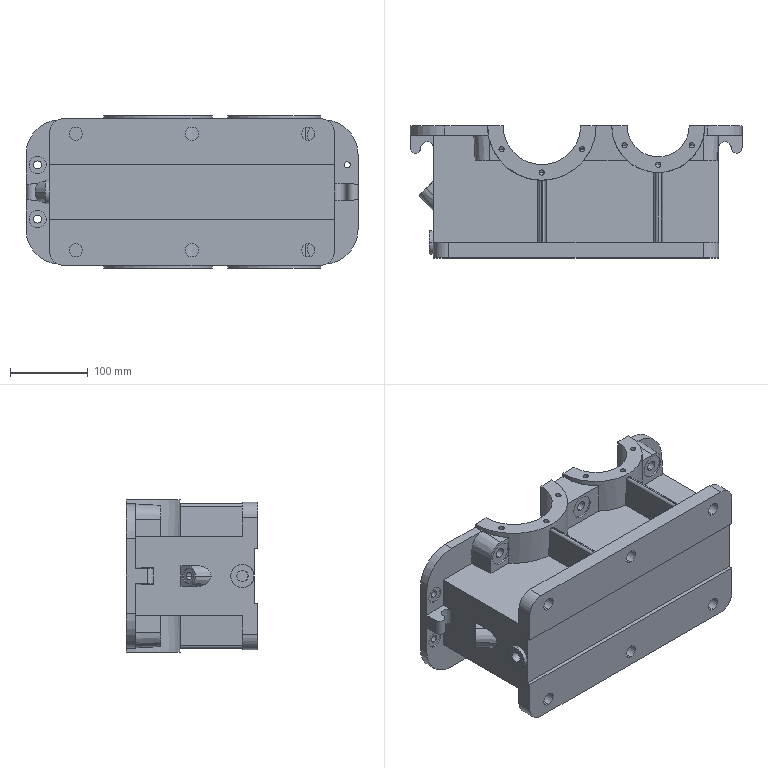Part | SolidWorks | features ICE 21, 3DProfileFeature 10, HoleWzd 10, MirrorPattern 10, Draft 8, Fillet 8, CirPattern 2, Rib 2, Extrusion 1, LPattern 1 | 1 solid | 246 faces | box 428 x 170 x 196 mm | volume 3193437 mm3 | cylinder 120 | plane 94 | cone 32 | commonest cylinder face diameters 30 x26 6.8 x24 13 x12 17 x12 7 x8 8 x4